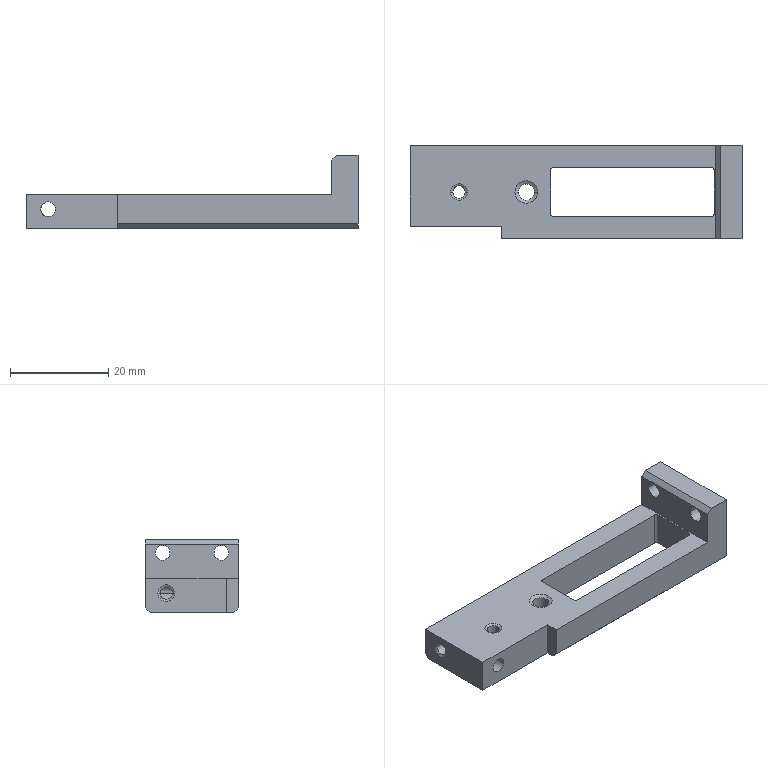Part | NX | 1 solid | 39 faces | box 67.7 x 19 x 15 mm | volume 6788 mm3 | plane 17 | cylinder 16 | cone 6 | commonest cylinder face diameters 3 x6 1 x4 2.5 x4 3.3 x2
STEP:
#1=CARTESIAN_POINT('',(-33.85,-7.,-3.5));
#2=VERTEX_POINT('',#1);
#3=CARTESIAN_POINT('',(-33.85,-7.,3.5));
#4=VERTEX_POINT('',#3);
#5=CARTESIAN_POINT('',(-33.85,-7.,0.));
#6=DIRECTION('',(0.,0.,1.));
#7=VECTOR('',#6,1000.);
#8=LINE('',#5,#7);
#9=EDGE_CURVE('',#2,#4,#8,.T.);
#10=ORIENTED_EDGE('',*,*,#9,.T.);
#11=CARTESIAN_POINT('',(-33.85,9.5,3.5));
#12=VERTEX_POINT('',#11);
#13=CARTESIAN_POINT('',(-33.85,0.,3.5));
#14=DIRECTION('',(0.,1.,0.));
#15=VECTOR('',#14,1000.);
#16=LINE('',#13,#15);
#17=EDGE_CURVE('',#4,#12,#16,.T.);
#18=ORIENTED_EDGE('',*,*,#17,.T.);
#19=CARTESIAN_POINT('',(-33.85,9.5,-2.5));
#20=VERTEX_POINT('',#19);
#21=CARTESIAN_POINT('',(-33.85,9.5,0.));
#22=DIRECTION('',(0.,0.,1.));
#23=VECTOR('',#22,1000.);
#24=LINE('',#21,#23);
#25=EDGE_CURVE('',#20,#12,#24,.T.);
#26=ORIENTED_EDGE('',*,*,#25,.F.);
#27=CARTESIAN_POINT('',(-33.85,8.5,-3.5));
#28=VERTEX_POINT('',#27);
#29=CARTESIAN_POINT('',(-33.85,12.,0.));
#30=DIRECTION('',(0.,0.7071,0.7071));
#31=VECTOR('',#30,1000.);
#32=LINE('',#29,#31);
#33=EDGE_CURVE('',#28,#20,#32,.T.);
#34=ORIENTED_EDGE('',*,*,#33,.F.);
#35=CARTESIAN_POINT('',(-33.85,0.,-3.5));
#36=DIRECTION('',(0.,1.,0.));
#37=VECTOR('',#36,1000.);
#38=LINE('',#35,#37);
#39=EDGE_CURVE('',#2,#28,#38,.T.);
#40=ORIENTED_EDGE('',*,*,#39,.F.);
#41=EDGE_LOOP('',(#10,#18,#26,#34,#40));
#42=FACE_BOUND('',#41,.T.);
#43=CARTESIAN_POINT('',(-33.85,6.95,0.5));
#44=VERTEX_POINT('',#43);
#45=CARTESIAN_POINT('',(-33.85,3.55,0.5));
#46=VERTEX_POINT('',#45);
#47=CARTESIAN_POINT('',(-33.85,5.25,0.5));
#48=DIRECTION('',(-1.,0.,0.));
#49=DIRECTION('',(0.,1.,0.));
#50=AXIS2_PLACEMENT_3D('',#47,#48,#49);
#51=CIRCLE('',#50,1.7);
#52=EDGE_CURVE('',#44,#46,#51,.T.);
#53=ORIENTED_EDGE('',*,*,#52,.F.);
#54=CARTESIAN_POINT('',(-33.85,5.25,0.5));
#55=DIRECTION('',(-1.,0.,0.));
#56=DIRECTION('',(0.,1.,0.));
#57=AXIS2_PLACEMENT_3D('',#54,#55,#56);
#58=CIRCLE('',#57,1.7);
#59=EDGE_CURVE('',#46,#44,#58,.T.);
#60=ORIENTED_EDGE('',*,*,#59,.F.);
#61=EDGE_LOOP('',(#53,#60));
#62=FACE_BOUND('',#61,.T.);
#63=CARTESIAN_POINT('',(-33.85,9.5,-3.5));
#64=DIRECTION('',(-1.,0.,0.));
#65=DIRECTION('',(0.,0.,1.));
#66=AXIS2_PLACEMENT_3D('',#63,#64,#65);
#67=PLANE('',#66);
#68=ADVANCED_FACE('',(#42,#62),#67,.T.);
#69=CARTESIAN_POINT('',(-15.15,-7.,-3.5));
#70=VERTEX_POINT('',#69);
#71=CARTESIAN_POINT('',(-15.15,-8.5,-3.5));
#72=VERTEX_POINT('',#71);
#73=CARTESIAN_POINT('',(-15.15,0.,-3.5));
#74=DIRECTION('',(0.,-1.,0.));
#75=VECTOR('',#74,1000.);
#76=LINE('',#73,#75);
#77=EDGE_CURVE('',#70,#72,#76,.T.);
#78=ORIENTED_EDGE('',*,*,#77,.T.);
#79=CARTESIAN_POINT('',(-15.15,-9.5,-2.5));
#80=VERTEX_POINT('',#79);
#81=CARTESIAN_POINT('',(-15.15,-9.5,-2.5));
#82=DIRECTION('',(0.,0.7071,-0.7071));
#83=VECTOR('',#82,1000.);
#84=LINE('',#81,#83);
#85=EDGE_CURVE('',#80,#72,#84,.T.);
#86=ORIENTED_EDGE('',*,*,#85,.F.);
#87=CARTESIAN_POINT('',(-15.15,-9.5,3.5));
#88=VERTEX_POINT('',#87);
#89=CARTESIAN_POINT('',(-15.15,-9.5,3.5));
#90=DIRECTION('',(0.,0.,-1.));
#91=VECTOR('',#90,1000.);
#92=LINE('',#89,#91);
#93=EDGE_CURVE('',#88,#80,#92,.T.);
#94=ORIENTED_EDGE('',*,*,#93,.F.);
#95=CARTESIAN_POINT('',(-15.15,-7.,3.5));
#96=VERTEX_POINT('',#95);
#97=CARTESIAN_POINT('',(-15.15,0.,3.5));
#98=DIRECTION('',(0.,-1.,0.));
#99=VECTOR('',#98,1000.);
#100=LINE('',#97,#99);
#101=EDGE_CURVE('',#96,#88,#100,.T.);
#102=ORIENTED_EDGE('',*,*,#101,.F.);
#103=CARTESIAN_POINT('',(-15.15,-7.,-3.5));
#104=DIRECTION('',(0.,0.,1.));
#105=VECTOR('',#104,1000.);
#106=LINE('',#103,#105);
#107=EDGE_CURVE('',#70,#96,#106,.T.);
#108=ORIENTED_EDGE('',*,*,#107,.F.);
#109=EDGE_LOOP('',(#78,#86,#94,#102,#108));
#110=FACE_BOUND('',#109,.T.);
#111=CARTESIAN_POINT('',(-15.15,-9.5,3.5));
#112=DIRECTION('',(1.,0.,0.));
#113=DIRECTION('',(0.,1.,0.));
#114=AXIS2_PLACEMENT_3D('',#111,#112,#113);
#115=PLANE('',#114);
#116=ADVANCED_FACE('',(#110),#115,.F.);
#117=CARTESIAN_POINT('',(33.85,8.5,-3.5));
#118=VERTEX_POINT('',#117);
#119=CARTESIAN_POINT('',(0.,8.5,-3.5));
#120=DIRECTION('',(1.,0.,0.));
#121=VECTOR('',#120,1000.);
#122=LINE('',#119,#121);
#123=EDGE_CURVE('',#28,#118,#122,.T.);
#124=ORIENTED_EDGE('',*,*,#123,.T.);
#125=CARTESIAN_POINT('',(33.85,-8.5,-3.5));
#126=VERTEX_POINT('',#125);
#127=CARTESIAN_POINT('',(33.85,0.,-3.5));
#128=DIRECTION('',(0.,1.,0.));
#129=VECTOR('',#128,1000.);
#130=LINE('',#127,#129);
#131=EDGE_CURVE('',#126,#118,#130,.T.);
#132=ORIENTED_EDGE('',*,*,#131,.F.);
#133=CARTESIAN_POINT('',(0.,-8.5,-3.5));
#134=DIRECTION('',(-1.,0.,0.));
#135=VECTOR('',#134,1000.);
#136=LINE('',#133,#135);
#137=EDGE_CURVE('',#126,#72,#136,.T.);
#138=ORIENTED_EDGE('',*,*,#137,.T.);
#139=ORIENTED_EDGE('',*,*,#77,.F.);
#140=CARTESIAN_POINT('',(0.,-7.,-3.5));
#141=DIRECTION('',(1.,0.,0.));
#142=VECTOR('',#141,1000.);
#143=LINE('',#140,#142);
#144=EDGE_CURVE('',#2,#70,#143,.T.);
#145=ORIENTED_EDGE('',*,*,#144,.F.);
#146=ORIENTED_EDGE('',*,*,#39,.T.);
#147=EDGE_LOOP('',(#124,#132,#138,#139,#145,#146));
#148=FACE_BOUND('',#147,.T.);
#149=CARTESIAN_POINT('',(27.65,-5.,-3.5));
#150=VERTEX_POINT('',#149);
#151=CARTESIAN_POINT('',(-4.65,-5.,-3.5));
#152=VERTEX_POINT('',#151);
#153=CARTESIAN_POINT('',(0.,-5.,-3.5));
#154=DIRECTION('',(-1.,0.,0.));
#155=VECTOR('',#154,1000.);
#156=LINE('',#153,#155);
#157=EDGE_CURVE('',#150,#152,#156,.T.);
#158=ORIENTED_EDGE('',*,*,#157,.F.);
#159=CARTESIAN_POINT('',(28.15,-4.5,-3.5));
#160=VERTEX_POINT('',#159);
#161=CARTESIAN_POINT('',(27.65,-4.5,-3.5));
#162=DIRECTION('',(0.,0.,1.));
#163=DIRECTION('',(0.,1.,0.));
#164=AXIS2_PLACEMENT_3D('',#161,#162,#163);
#165=CIRCLE('',#164,0.5);
#166=EDGE_CURVE('',#150,#160,#165,.T.);
#167=ORIENTED_EDGE('',*,*,#166,.T.);
#168=CARTESIAN_POINT('',(28.15,4.5,-3.5));
#169=VERTEX_POINT('',#168);
#170=CARTESIAN_POINT('',(28.15,0.,-3.5));
#171=DIRECTION('',(0.,-1.,0.));
#172=VECTOR('',#171,1000.);
#173=LINE('',#170,#172);
#174=EDGE_CURVE('',#169,#160,#173,.T.);
#175=ORIENTED_EDGE('',*,*,#174,.F.);
#176=CARTESIAN_POINT('',(27.65,5.,-3.5));
#177=VERTEX_POINT('',#176);
#178=CARTESIAN_POINT('',(27.65,4.5,-3.5));
#179=DIRECTION('',(0.,0.,1.));
#180=DIRECTION('',(0.,1.,0.));
#181=AXIS2_PLACEMENT_3D('',#178,#179,#180);
#182=CIRCLE('',#181,0.5);
#183=EDGE_CURVE('',#169,#177,#182,.T.);
#184=ORIENTED_EDGE('',*,*,#183,.T.);
#185=CARTESIAN_POINT('',(-4.65,5.,-3.5));
#186=VERTEX_POINT('',#185);
#187=CARTESIAN_POINT('',(0.,5.,-3.5));
#188=DIRECTION('',(1.,0.,0.));
#189=VECTOR('',#188,1000.);
#190=LINE('',#187,#189);
#191=EDGE_CURVE('',#186,#177,#190,.T.);
#192=ORIENTED_EDGE('',*,*,#191,.F.);
#193=CARTESIAN_POINT('',(-5.15,4.5,-3.5));
#194=VERTEX_POINT('',#193);
#195=CARTESIAN_POINT('',(-4.65,4.5,-3.5));
#196=DIRECTION('',(0.,0.,1.));
#197=DIRECTION('',(0.,1.,0.));
#198=AXIS2_PLACEMENT_3D('',#195,#196,#197);
#199=CIRCLE('',#198,0.5);
#200=EDGE_CURVE('',#186,#194,#199,.T.);
#201=ORIENTED_EDGE('',*,*,#200,.T.);
#202=CARTESIAN_POINT('',(-5.15,-4.5,-3.5));
#203=VERTEX_POINT('',#202);
#204=CARTESIAN_POINT('',(-5.15,0.,-3.5));
#205=DIRECTION('',(0.,1.,0.));
#206=VECTOR('',#205,1000.);
#207=LINE('',#204,#206);
#208=EDGE_CURVE('',#203,#194,#207,.T.);
#209=ORIENTED_EDGE('',*,*,#208,.F.);
#210=CARTESIAN_POINT('',(-4.65,-4.5,-3.5));
#211=DIRECTION('',(0.,0.,1.));
#212=DIRECTION('',(0.,1.,0.));
#213=AXIS2_PLACEMENT_3D('',#210,#211,#212);
#214=CIRCLE('',#213,0.5);
#215=EDGE_CURVE('',#203,#152,#214,.T.);
#216=ORIENTED_EDGE('',*,*,#215,.T.);
#217=EDGE_LOOP('',(#158,#167,#175,#184,#192,#201,#209,#216));
#218=FACE_BOUND('',#217,.T.);
#219=CARTESIAN_POINT('',(-22.6,0.,-3.5));
#220=VERTEX_POINT('',#219);
#221=CARTESIAN_POINT('',(-25.1,0.,-3.5));
#222=VERTEX_POINT('',#221);
#223=CARTESIAN_POINT('',(-23.85,0.,-3.5));
#224=DIRECTION('',(0.,0.,1.));
#225=DIRECTION('',(1.,0.,0.));
#226=AXIS2_PLACEMENT_3D('',#223,#224,#225);
#227=CIRCLE('',#226,1.25);
#228=EDGE_CURVE('',#220,#222,#227,.T.);
#229=ORIENTED_EDGE('',*,*,#228,.T.);
#230=CARTESIAN_POINT('',(-23.85,0.,-3.5));
#231=DIRECTION('',(0.,0.,1.));
#232=DIRECTION('',(1.,0.,0.));
#233=AXIS2_PLACEMENT_3D('',#230,#231,#232);
#234=CIRCLE('',#233,1.25);
#235=EDGE_CURVE('',#222,#220,#234,.T.);
#236=ORIENTED_EDGE('',*,*,#235,.T.);
#237=EDGE_LOOP('',(#229,#236));
#238=FACE_BOUND('',#237,.T.);
#239=CARTESIAN_POINT('',(-11.8,0.,-3.5));
#240=VERTEX_POINT('',#239);
#241=CARTESIAN_POINT('',(-8.5,0.,-3.5));
#242=VERTEX_POINT('',#241);
#243=CARTESIAN_POINT('',(-10.15,0.,-3.5));
#244=DIRECTION('',(0.,0.,1.));
#245=DIRECTION('',(1.,0.,0.));
#246=AXIS2_PLACEMENT_3D('',#243,#244,#245);
#247=CIRCLE('',#246,1.65);
#248=EDGE_CURVE('',#240,#242,#247,.T.);
#249=ORIENTED_EDGE('',*,*,#248,.T.);
#250=CARTESIAN_POINT('',(-10.15,0.,-3.5));
#251=DIRECTION('',(0.,0.,1.));
#252=DIRECTION('',(1.,0.,0.));
#253=AXIS2_PLACEMENT_3D('',#250,#251,#252);
#254=CIRCLE('',#253,1.65);
#255=EDGE_CURVE('',#242,#240,#254,.T.);
#256=ORIENTED_EDGE('',*,*,#255,.T.);
#257=EDGE_LOOP('',(#249,#256));
#258=FACE_BOUND('',#257,.T.);
#259=CARTESIAN_POINT('',(0.,0.,-3.5));
#260=DIRECTION('',(0.,0.,1.));
#261=DIRECTION('',(1.,0.,0.));
#262=AXIS2_PLACEMENT_3D('',#259,#260,#261);
#263=PLANE('',#262);
#264=ADVANCED_FACE('',(#148,#218,#238,#258),#263,.F.);
#265=CARTESIAN_POINT('',(28.5,9.5,3.5));
#266=VERTEX_POINT('',#265);
#267=CARTESIAN_POINT('',(28.5,-9.5,3.5));
#268=VERTEX_POINT('',#267);
#269=CARTESIAN_POINT('',(28.5,0.,3.5));
#270=DIRECTION('',(0.,-1.,0.));
#271=VECTOR('',#270,1000.);
#272=LINE('',#269,#271);
#273=EDGE_CURVE('',#266,#268,#272,.T.);
#274=ORIENTED_EDGE('',*,*,#273,.T.);
#275=CARTESIAN_POINT('',(28.5,-9.5,10.5));
#276=VERTEX_POINT('',#275);
#277=CARTESIAN_POINT('',(28.5,-9.5,0.));
#278=DIRECTION('',(0.,0.,-1.));
#279=VECTOR('',#278,1000.);
#280=LINE('',#277,#279);
#281=EDGE_CURVE('',#276,#268,#280,.T.);
#282=ORIENTED_EDGE('',*,*,#281,.F.);
#283=CARTESIAN_POINT('',(28.5,9.5,10.5));
#284=VERTEX_POINT('',#283);
#285=CARTESIAN_POINT('',(28.5,0.,10.5));
#286=DIRECTION('',(0.,1.,0.));
#287=VECTOR('',#286,1000.);
#288=LINE('',#285,#287);
#289=EDGE_CURVE('',#276,#284,#288,.T.);
#290=ORIENTED_EDGE('',*,*,#289,.T.);
#291=CARTESIAN_POINT('',(28.5,9.5,0.));
#292=DIRECTION('',(0.,0.,1.));
#293=VECTOR('',#292,1000.);
#294=LINE('',#291,#293);
#295=EDGE_CURVE('',#266,#284,#294,.T.);
#296=ORIENTED_EDGE('',*,*,#295,.F.);
#297=EDGE_LOOP('',(#274,#282,#290,#296));
#298=FACE_BOUND('',#297,.T.);
#299=CARTESIAN_POINT('',(28.5,-4.5,8.73));
#300=VERTEX_POINT('',#299);
#301=CARTESIAN_POINT('',(28.5,-7.5,8.73));
#302=VERTEX_POINT('',#301);
#303=CARTESIAN_POINT('',(28.5,-6.,8.73));
#304=DIRECTION('',(1.,0.,0.));
#305=DIRECTION('',(0.,1.,0.));
#306=AXIS2_PLACEMENT_3D('',#303,#304,#305);
#307=CIRCLE('',#306,1.5);
#308=EDGE_CURVE('',#300,#302,#307,.T.);
#309=ORIENTED_EDGE('',*,*,#308,.T.);
#310=CARTESIAN_POINT('',(28.5,-6.,8.73));
#311=DIRECTION('',(1.,0.,0.));
#312=DIRECTION('',(0.,1.,0.));
#313=AXIS2_PLACEMENT_3D('',#310,#311,#312);
#314=CIRCLE('',#313,1.5);
#315=EDGE_CURVE('',#302,#300,#314,.T.);
#316=ORIENTED_EDGE('',*,*,#315,.T.);
#317=EDGE_LOOP('',(#309,#316));
#318=FACE_BOUND('',#317,.T.);
#319=CARTESIAN_POINT('',(28.5,7.5,8.73));
#320=VERTEX_POINT('',#319);
#321=CARTESIAN_POINT('',(28.5,4.5,8.73));
#322=VERTEX_POINT('',#321);
#323=CARTESIAN_POINT('',(28.5,6.,8.73));
#324=DIRECTION('',(1.,0.,0.));
#325=DIRECTION('',(0.,1.,0.));
#326=AXIS2_PLACEMENT_3D('',#323,#324,#325);
#327=CIRCLE('',#326,1.5);
#328=EDGE_CURVE('',#320,#322,#327,.T.);
#329=ORIENTED_EDGE('',*,*,#328,.T.);
#330=CARTESIAN_POINT('',(28.5,6.,8.73));
#331=DIRECTION('',(1.,0.,0.));
#332=DIRECTION('',(0.,1.,0.));
#333=AXIS2_PLACEMENT_3D('',#330,#331,#332);
#334=CIRCLE('',#333,1.5);
#335=EDGE_CURVE('',#322,#320,#334,.T.);
#336=ORIENTED_EDGE('',*,*,#335,.T.);
#337=EDGE_LOOP('',(#329,#336));
#338=FACE_BOUND('',#337,.T.);
#339=CARTESIAN_POINT('',(28.5,9.5,3.5));
#340=DIRECTION('',(-1.,0.,0.));
#341=DIRECTION('',(0.,0.,1.));
#342=AXIS2_PLACEMENT_3D('',#339,#340,#341);
#343=PLANE('',#342);
#344=ADVANCED_FACE('',(#298,#318,#338),#343,.T.);
#345=ORIENTED_EDGE('',*,*,#101,.T.);
#346=CARTESIAN_POINT('',(0.,-9.5,3.5));
#347=DIRECTION('',(-1.,0.,0.));
#348=VECTOR('',#347,1000.);
#349=LINE('',#346,#348);
#350=EDGE_CURVE('',#268,#88,#349,.T.);
#351=ORIENTED_EDGE('',*,*,#350,.F.);
#352=ORIENTED_EDGE('',*,*,#273,.F.);
#353=CARTESIAN_POINT('',(0.,9.5,3.5));
#354=DIRECTION('',(1.,0.,0.));
#355=VECTOR('',#354,1000.);
#356=LINE('',#353,#355);
#357=EDGE_CURVE('',#12,#266,#356,.T.);
#358=ORIENTED_EDGE('',*,*,#357,.F.);
#359=ORIENTED_EDGE('',*,*,#17,.F.);
#360=CARTESIAN_POINT('',(0.,-7.,3.5));
#361=DIRECTION('',(1.,0.,0.));
#362=VECTOR('',#361,1000.);
#363=LINE('',#360,#362);
#364=EDGE_CURVE('',#4,#96,#363,.T.);
#365=ORIENTED_EDGE('',*,*,#364,.T.);
#366=EDGE_LOOP('',(#345,#351,#352,#358,#359,#365));
#367=FACE_BOUND('',#366,.T.);
#368=CARTESIAN_POINT('',(27.65,-5.,3.5));
#369=VERTEX_POINT('',#368);
#370=CARTESIAN_POINT('',(-4.65,-5.,3.5));
#371=VERTEX_POINT('',#370);
#372=CARTESIAN_POINT('',(0.,-5.,3.5));
#373=DIRECTION('',(-1.,0.,0.));
#374=VECTOR('',#373,1000.);
#375=LINE('',#372,#374);
#376=EDGE_CURVE('',#369,#371,#375,.T.);
#377=ORIENTED_EDGE('',*,*,#376,.T.);
#378=CARTESIAN_POINT('',(-5.15,-4.5,3.5));
#379=VERTEX_POINT('',#378);
#380=CARTESIAN_POINT('',(-4.65,-4.5,3.5));
#381=DIRECTION('',(0.,0.,1.));
#382=DIRECTION('',(0.,1.,0.));
#383=AXIS2_PLACEMENT_3D('',#380,#381,#382);
#384=CIRCLE('',#383,0.5);
#385=EDGE_CURVE('',#379,#371,#384,.T.);
#386=ORIENTED_EDGE('',*,*,#385,.F.);
#387=CARTESIAN_POINT('',(-5.15,4.5,3.5));
#388=VERTEX_POINT('',#387);
#389=CARTESIAN_POINT('',(-5.15,0.,3.5));
#390=DIRECTION('',(0.,1.,0.));
#391=VECTOR('',#390,1000.);
#392=LINE('',#389,#391);
#393=EDGE_CURVE('',#379,#388,#392,.T.);
#394=ORIENTED_EDGE('',*,*,#393,.T.);
#395=CARTESIAN_POINT('',(-4.65,5.,3.5));
#396=VERTEX_POINT('',#395);
#397=CARTESIAN_POINT('',(-4.65,4.5,3.5));
#398=DIRECTION('',(0.,0.,1.));
#399=DIRECTION('',(0.,1.,0.));
#400=AXIS2_PLACEMENT_3D('',#397,#398,#399);
#401=CIRCLE('',#400,0.5);
#402=EDGE_CURVE('',#396,#388,#401,.T.);
#403=ORIENTED_EDGE('',*,*,#402,.F.);
#404=CARTESIAN_POINT('',(27.65,5.,3.5));
#405=VERTEX_POINT('',#404);
#406=CARTESIAN_POINT('',(0.,5.,3.5));
#407=DIRECTION('',(1.,0.,0.));
#408=VECTOR('',#407,1000.);
#409=LINE('',#406,#408);
#410=EDGE_CURVE('',#396,#405,#409,.T.);
#411=ORIENTED_EDGE('',*,*,#410,.T.);
#412=CARTESIAN_POINT('',(28.15,4.5,3.5));
#413=VERTEX_POINT('',#412);
#414=CARTESIAN_POINT('',(27.65,4.5,3.5));
#415=DIRECTION('',(0.,0.,1.));
#416=DIRECTION('',(0.,1.,0.));
#417=AXIS2_PLACEMENT_3D('',#414,#415,#416);
#418=CIRCLE('',#417,0.5);
#419=EDGE_CURVE('',#413,#405,#418,.T.);
#420=ORIENTED_EDGE('',*,*,#419,.F.);
#421=CARTESIAN_POINT('',(28.15,-4.5,3.5));
#422=VERTEX_POINT('',#421);
#423=CARTESIAN_POINT('',(28.15,0.,3.5));
#424=DIRECTION('',(0.,-1.,0.));
#425=VECTOR('',#424,1000.);
#426=LINE('',#423,#425);
#427=EDGE_CURVE('',#413,#422,#426,.T.);
#428=ORIENTED_EDGE('',*,*,#427,.T.);
#429=CARTESIAN_POINT('',(27.65,-4.5,3.5));
#430=DIRECTION('',(0.,0.,1.));
#431=DIRECTION('',(0.,1.,0.));
#432=AXIS2_PLACEMENT_3D('',#429,#430,#431);
#433=CIRCLE('',#432,0.5);
#434=EDGE_CURVE('',#369,#422,#433,.T.);
#435=ORIENTED_EDGE('',*,*,#434,.F.);
#436=EDGE_LOOP('',(#377,#386,#394,#403,#411,#420,#428,#435));
#437=FACE_BOUND('',#436,.T.);
#438=CARTESIAN_POINT('',(-12.465,0.,3.5));
#439=VERTEX_POINT('',#438);
#440=CARTESIAN_POINT('',(-7.835,0.,3.5));
#441=VERTEX_POINT('',#440);
#442=CARTESIAN_POINT('',(-10.15,0.,3.5));
#443=DIRECTION('',(0.,0.,1.));
#444=DIRECTION('',(1.,0.,0.));
#445=AXIS2_PLACEMENT_3D('',#442,#443,#444);
#446=CIRCLE('',#445,2.315);
#447=EDGE_CURVE('',#439,#441,#446,.T.);
#448=ORIENTED_EDGE('',*,*,#447,.F.);
#449=CARTESIAN_POINT('',(-10.15,0.,3.5));
#450=DIRECTION('',(0.,0.,1.));
#451=DIRECTION('',(1.,0.,0.));
#452=AXIS2_PLACEMENT_3D('',#449,#450,#451);
#453=CIRCLE('',#452,2.315);
#454=EDGE_CURVE('',#441,#439,#453,.T.);
#455=ORIENTED_EDGE('',*,*,#454,.F.);
#456=EDGE_LOOP('',(#448,#455));
#457=FACE_BOUND('',#456,.T.);
#458=CARTESIAN_POINT('',(-22.15,0.,3.5));
#459=VERTEX_POINT('',#458);
#460=CARTESIAN_POINT('',(-25.55,0.,3.5));
#461=VERTEX_POINT('',#460);
#462=CARTESIAN_POINT('',(-23.85,0.,3.5));
#463=DIRECTION('',(0.,0.,1.));
#464=DIRECTION('',(1.,0.,0.));
#465=AXIS2_PLACEMENT_3D('',#462,#463,#464);
#466=CIRCLE('',#465,1.7);
#467=EDGE_CURVE('',#459,#461,#466,.T.);
#468=ORIENTED_EDGE('',*,*,#467,.F.);
#469=CARTESIAN_POINT('',(-23.85,0.,3.5));
#470=DIRECTION('',(0.,0.,1.));
#471=DIRECTION('',(1.,0.,0.));
#472=AXIS2_PLACEMENT_3D('',#469,#470,#471);
#473=CIRCLE('',#472,1.7);
#474=EDGE_CURVE('',#461,#459,#473,.T.);
#475=ORIENTED_EDGE('',*,*,#474,.F.);
#476=EDGE_LOOP('',(#468,#475));
#477=FACE_BOUND('',#476,.T.);
#478=CARTESIAN_POINT('',(0.,0.,3.5));
#479=DIRECTION('',(0.,0.,1.));
#480=DIRECTION('',(1.,0.,0.));
#481=AXIS2_PLACEMENT_3D('',#478,#479,#480);
#482=PLANE('',#481);
#483=ADVANCED_FACE('',(#367,#437,#457,#477),#482,.T.);
#484=CARTESIAN_POINT('',(-30.85,6.5,0.5));
#485=VERTEX_POINT('',#484);
#486=CARTESIAN_POINT('',(-30.85,4.,0.5));
#487=VERTEX_POINT('',#486);
#488=CARTESIAN_POINT('',(-30.85,6.5,0.5));
#489=CARTESIAN_POINT('',(-30.85,6.5,0.6667));
#490=CARTESIAN_POINT('',(-30.788,6.424,0.9601));
#491=CARTESIAN_POINT('',(-30.695,6.313,1.179));
#492=CARTESIAN_POINT('',(-30.552,6.12,1.4));
#493=CARTESIAN_POINT('',(-30.532,6.094,1.425));
#494=CARTESIAN_POINT('',(-30.389,5.883,1.59));
#495=CARTESIAN_POINT('',(-30.285,5.699,1.674));
#496=CARTESIAN_POINT('',(-30.109,5.25,1.801));
#497=CARTESIAN_POINT('',(-30.284,4.802,1.674));
#498=CARTESIAN_POINT('',(-30.39,4.616,1.589));
#499=CARTESIAN_POINT('',(-30.53,4.408,1.427));
#500=CARTESIAN_POINT('',(-30.553,4.379,1.399));
#501=CARTESIAN_POINT('',(-30.695,4.187,1.18));
#502=CARTESIAN_POINT('',(-30.788,4.076,0.9605));
#503=CARTESIAN_POINT('',(-30.85,4.,0.6669));
#504=CARTESIAN_POINT('',(-30.85,4.,0.5));
#505=B_SPLINE_CURVE_WITH_KNOTS('',3,(#488,#489,#490,#491,#492,#493,#494,#495,#496,#497,#498,#499,#500,#501,#502,#503,#504),.UNSPECIFIED.,.F.,.F.,(4,1,1,1,1,1,1,1,1,1,1,1,1,1,4),(0.,0.125,0.1875,0.25,0.2812,0.3125,0.375,0.5,0.625,0.6875,0.7188,0.75,0.8125,0.875,1.),.UNSPECIFIED.);
#506=EDGE_CURVE('',#485,#487,#505,.T.);
#507=ORIENTED_EDGE('',*,*,#506,.T.);
#508=CARTESIAN_POINT('',(-33.59,4.,0.5));
#509=VERTEX_POINT('',#508);
#510=CARTESIAN_POINT('',(-33.85,4.,0.5));
#511=DIRECTION('',(-1.,0.,0.));
#512=VECTOR('',#511,1000.);
#513=LINE('',#510,#512);
#514=EDGE_CURVE('',#487,#509,#513,.T.);
#515=ORIENTED_EDGE('',*,*,#514,.T.);
#516=CARTESIAN_POINT('',(-33.59,6.5,0.5));
#517=VERTEX_POINT('',#516);
#518=CARTESIAN_POINT('',(-33.59,5.25,0.5));
#519=DIRECTION('',(-1.,0.,0.));
#520=DIRECTION('',(0.,1.,0.));
#521=AXIS2_PLACEMENT_3D('',#518,#519,#520);
#522=CIRCLE('',#521,1.25);
#523=EDGE_CURVE('',#509,#517,#522,.T.);
#524=ORIENTED_EDGE('',*,*,#523,.T.);
#525=CARTESIAN_POINT('',(-33.85,6.5,0.5));
#526=DIRECTION('',(-1.,0.,0.));
#527=VECTOR('',#526,1000.);
#528=LINE('',#525,#527);
#529=EDGE_CURVE('',#485,#517,#528,.T.);
#530=ORIENTED_EDGE('',*,*,#529,.F.);
#531=EDGE_LOOP('',(#507,#515,#524,#530));
#532=FACE_BOUND('',#531,.T.);
#533=CARTESIAN_POINT('',(-33.85,5.25,0.5));
#534=DIRECTION('',(-1.,0.,0.));
#535=DIRECTION('',(0.,1.,0.));
#536=AXIS2_PLACEMENT_3D('',#533,#534,#535);
#537=CYLINDRICAL_SURFACE('',#536,1.25);
#538=ADVANCED_FACE('',(#532),#537,.F.);
#539=ORIENTED_EDGE('',*,*,#52,.T.);
#540=CARTESIAN_POINT('',(-33.59,4.,0.5));
#541=DIRECTION('',(-0.5,-0.866,0.));
#542=VECTOR('',#541,1000.);
#543=LINE('',#540,#542);
#544=EDGE_CURVE('',#46,#509,#543,.F.);
#545=ORIENTED_EDGE('',*,*,#544,.T.);
#546=CARTESIAN_POINT('',(-33.59,5.25,0.5));
#547=DIRECTION('',(-1.,0.,0.));
#548=DIRECTION('',(0.,1.,0.));
#549=AXIS2_PLACEMENT_3D('',#546,#547,#548);
#550=CIRCLE('',#549,1.25);
#551=EDGE_CURVE('',#517,#509,#550,.T.);
#552=ORIENTED_EDGE('',*,*,#551,.F.);
#553=CARTESIAN_POINT('',(-33.59,6.5,0.5));
#554=DIRECTION('',(-0.5,0.866,0.));
#555=VECTOR('',#554,1000.);
#556=LINE('',#553,#555);
#557=EDGE_CURVE('',#44,#517,#556,.F.);
#558=ORIENTED_EDGE('',*,*,#557,.F.);
#559=EDGE_LOOP('',(#539,#545,#552,#558));
#560=FACE_BOUND('',#559,.T.);
#561=CARTESIAN_POINT('',(-33.59,5.25,0.5));
#562=DIRECTION('',(-1.,0.,0.));
#563=DIRECTION('',(0.,1.,0.));
#564=AXIS2_PLACEMENT_3D('',#561,#562,#563);
#565=CONICAL_SURFACE('',#564,1.25,1.047);
#566=ADVANCED_FACE('',(#560),#565,.F.);
#567=CARTESIAN_POINT('',(33.85,9.5,-2.5));
#568=VERTEX_POINT('',#567);
#569=CARTESIAN_POINT('',(0.,9.5,-2.5));
#570=DIRECTION('',(1.,0.,0.));
#571=VECTOR('',#570,1000.);
#572=LINE('',#569,#571);
#573=EDGE_CURVE('',#20,#568,#572,.T.);
#574=ORIENTED_EDGE('',*,*,#573,.F.);
#575=ORIENTED_EDGE('',*,*,#25,.T.);
#576=ORIENTED_EDGE('',*,*,#357,.T.);
#577=ORIENTED_EDGE('',*,*,#295,.T.);
#578=CARTESIAN_POINT('',(29.5,9.5,11.5));
#579=VERTEX_POINT('',#578);
#580=CARTESIAN_POINT('',(18.,9.5,0.));
#581=DIRECTION('',(0.7071,0.,0.7071));
#582=VECTOR('',#581,1000.);
#583=LINE('',#580,#582);
#584=EDGE_CURVE('',#284,#579,#583,.T.);
#585=ORIENTED_EDGE('',*,*,#584,.T.);
#586=CARTESIAN_POINT('',(33.85,9.5,11.5));
#587=VERTEX_POINT('',#586);
#588=CARTESIAN_POINT('',(0.,9.5,11.5));
#589=DIRECTION('',(-1.,0.,0.));
#590=VECTOR('',#589,1000.);
#591=LINE('',#588,#590);
#592=EDGE_CURVE('',#587,#579,#591,.T.);
#593=ORIENTED_EDGE('',*,*,#592,.F.);
#594=CARTESIAN_POINT('',(33.85,9.5,0.));
#595=DIRECTION('',(0.,0.,-1.));
#596=VECTOR('',#595,1000.);
#597=LINE('',#594,#596);
#598=EDGE_CURVE('',#587,#568,#597,.T.);
#599=ORIENTED_EDGE('',*,*,#598,.T.);
#600=EDGE_LOOP('',(#574,#575,#576,#577,#585,#593,#599));
#601=FACE_BOUND('',#600,.T.);
#602=CARTESIAN_POINT('',(-30.85,9.5,0.5));
#603=VERTEX_POINT('',#602);
#604=CARTESIAN_POINT('',(-27.85,9.5,0.5));
#605=VERTEX_POINT('',#604);
#606=CARTESIAN_POINT('',(-29.35,9.5,0.5));
#607=DIRECTION('',(0.,1.,0.));
#608=DIRECTION('',(-1.,0.,0.));
#609=AXIS2_PLACEMENT_3D('',#606,#607,#608);
#610=CIRCLE('',#609,1.5);
#611=EDGE_CURVE('',#603,#605,#610,.T.);
#612=ORIENTED_EDGE('',*,*,#611,.F.);
#613=CARTESIAN_POINT('',(-29.35,9.5,0.5));
#614=DIRECTION('',(0.,1.,0.));
#615=DIRECTION('',(-1.,0.,0.));
#616=AXIS2_PLACEMENT_3D('',#613,#614,#615);
#617=CIRCLE('',#616,1.5);
#618=EDGE_CURVE('',#605,#603,#617,.T.);
#619=ORIENTED_EDGE('',*,*,#618,.F.);
#620=EDGE_LOOP('',(#612,#619));
#621=FACE_BOUND('',#620,.T.);
#622=CARTESIAN_POINT('',(33.85,9.5,-3.5));
#623=DIRECTION('',(0.,1.,0.));
#624=DIRECTION('',(1.,0.,0.));
#625=AXIS2_PLACEMENT_3D('',#622,#623,#624);
#626=PLANE('',#625);
#627=ADVANCED_FACE('',(#601,#621),#626,.T.);
#628=ORIENTED_EDGE('',*,*,#93,.T.);
#629=CARTESIAN_POINT('',(33.85,-9.5,-2.5));
#630=VERTEX_POINT('',#629);
#631=CARTESIAN_POINT('',(33.85,-9.5,-2.5));
#632=DIRECTION('',(-1.,0.,0.));
#633=VECTOR('',#632,1000.);
#634=LINE('',#631,#633);
#635=EDGE_CURVE('',#630,#80,#634,.T.);
#636=ORIENTED_EDGE('',*,*,#635,.F.);
#637=CARTESIAN_POINT('',(33.85,-9.5,11.5));
#638=VERTEX_POINT('',#637);
#639=CARTESIAN_POINT('',(33.85,-9.5,0.));
#640=DIRECTION('',(0.,0.,1.));
#641=VECTOR('',#640,1000.);
#642=LINE('',#639,#641);
#643=EDGE_CURVE('',#630,#638,#642,.T.);
#644=ORIENTED_EDGE('',*,*,#643,.T.);
#645=CARTESIAN_POINT('',(29.5,-9.5,11.5));
#646=VERTEX_POINT('',#645);
#647=CARTESIAN_POINT('',(33.85,-9.5,11.5));
#648=DIRECTION('',(-1.,0.,0.));
#649=VECTOR('',#648,1000.);
#650=LINE('',#647,#649);
#651=EDGE_CURVE('',#638,#646,#650,.T.);
#652=ORIENTED_EDGE('',*,*,#651,.T.);
#653=CARTESIAN_POINT('',(28.5,-9.5,10.5));
#654=DIRECTION('',(0.7071,0.,0.7071));
#655=VECTOR('',#654,1000.);
#656=LINE('',#653,#655);
#657=EDGE_CURVE('',#276,#646,#656,.T.);
#658=ORIENTED_EDGE('',*,*,#657,.F.);
#659=ORIENTED_EDGE('',*,*,#281,.T.);
#660=ORIENTED_EDGE('',*,*,#350,.T.);
#661=EDGE_LOOP('',(#628,#636,#644,#652,#658,#659,#660));
#662=FACE_BOUND('',#661,.T.);
#663=CARTESIAN_POINT('',(-33.85,-9.5,-3.5));
#664=DIRECTION('',(0.,-1.,0.));
#665=DIRECTION('',(0.,0.,-1.));
#666=AXIS2_PLACEMENT_3D('',#663,#664,#665);
#667=PLANE('',#666);
#668=ADVANCED_FACE('',(#662),#667,.T.);
#669=ORIENTED_EDGE('',*,*,#598,.F.);
#670=CARTESIAN_POINT('',(33.85,0.,11.5));
#671=DIRECTION('',(0.,1.,0.));
#672=VECTOR('',#671,1000.);
#673=LINE('',#670,#672);
#674=EDGE_CURVE('',#638,#587,#673,.T.);
#675=ORIENTED_EDGE('',*,*,#674,.F.);
#676=ORIENTED_EDGE('',*,*,#643,.F.);
#677=CARTESIAN_POINT('',(33.85,-12.,0.));
#678=DIRECTION('',(0.,-0.7071,0.7071));
#679=VECTOR('',#678,1000.);
#680=LINE('',#677,#679);
#681=EDGE_CURVE('',#126,#630,#680,.T.);
#682=ORIENTED_EDGE('',*,*,#681,.F.);
#683=ORIENTED_EDGE('',*,*,#131,.T.);
#684=CARTESIAN_POINT('',(33.85,12.,0.));
#685=DIRECTION('',(0.,-0.7071,-0.7071));
#686=VECTOR('',#685,1000.);
#687=LINE('',#684,#686);
#688=EDGE_CURVE('',#568,#118,#687,.T.);
#689=ORIENTED_EDGE('',*,*,#688,.F.);
#690=EDGE_LOOP('',(#669,#675,#676,#682,#683,#689));
#691=FACE_BOUND('',#690,.T.);
#692=CARTESIAN_POINT('',(33.85,-4.5,8.73));
#693=VERTEX_POINT('',#692);
#694=CARTESIAN_POINT('',(33.85,-7.5,8.73));
#695=VERTEX_POINT('',#694);
#696=CARTESIAN_POINT('',(33.85,-6.,8.73));
#697=DIRECTION('',(1.,0.,0.));
#698=DIRECTION('',(0.,1.,0.));
#699=AXIS2_PLACEMENT_3D('',#696,#697,#698);
#700=CIRCLE('',#699,1.5);
#701=EDGE_CURVE('',#693,#695,#700,.T.);
#702=ORIENTED_EDGE('',*,*,#701,.F.);
#703=CARTESIAN_POINT('',(33.85,-6.,8.73));
#704=DIRECTION('',(1.,0.,0.));
#705=DIRECTION('',(0.,1.,0.));
#706=AXIS2_PLACEMENT_3D('',#703,#704,#705);
#707=CIRCLE('',#706,1.5);
#708=EDGE_CURVE('',#695,#693,#707,.T.);
#709=ORIENTED_EDGE('',*,*,#708,.F.);
#710=EDGE_LOOP('',(#702,#709));
#711=FACE_BOUND('',#710,.T.);
#712=CARTESIAN_POINT('',(33.85,4.5,8.73));
#713=VERTEX_POINT('',#712);
#714=CARTESIAN_POINT('',(33.85,7.5,8.73));
#715=VERTEX_POINT('',#714);
#716=CARTESIAN_POINT('',(33.85,6.,8.73));
#717=DIRECTION('',(1.,0.,0.));
#718=DIRECTION('',(0.,1.,0.));
#719=AXIS2_PLACEMENT_3D('',#716,#717,#718);
#720=CIRCLE('',#719,1.5);
#721=EDGE_CURVE('',#713,#715,#720,.T.);
#722=ORIENTED_EDGE('',*,*,#721,.F.);
#723=CARTESIAN_POINT('',(33.85,6.,8.73));
#724=DIRECTION('',(1.,0.,0.));
#725=DIRECTION('',(0.,1.,0.));
#726=AXIS2_PLACEMENT_3D('',#723,#724,#725);
#727=CIRCLE('',#726,1.5);
#728=EDGE_CURVE('',#715,#713,#727,.T.);
#729=ORIENTED_EDGE('',*,*,#728,.F.);
#730=EDGE_LOOP('',(#722,#729));
#731=FACE_BOUND('',#730,.T.);
#732=CARTESIAN_POINT('',(33.85,-9.5,-3.5));
#733=DIRECTION('',(1.,0.,0.));
#734=DIRECTION('',(0.,1.,0.));
#735=AXIS2_PLACEMENT_3D('',#732,#733,#734);
#736=PLANE('',#735);
#737=ADVANCED_FACE('',(#691,#711,#731),#736,.T.);
#738=ORIENTED_EDGE('',*,*,#248,.F.);
#739=CARTESIAN_POINT('',(-11.8,0.,3.116));
#740=VERTEX_POINT('',#739);
#741=CARTESIAN_POINT('',(-11.8,0.,3.5));
#742=DIRECTION('',(0.,0.,1.));
#743=VECTOR('',#742,1000.);
#744=LINE('',#741,#743);
#745=EDGE_CURVE('',#240,#740,#744,.T.);
#746=ORIENTED_EDGE('',*,*,#745,.T.);
#747=CARTESIAN_POINT('',(-8.5,0.,3.116));
#748=VERTEX_POINT('',#747);
#749=CARTESIAN_POINT('',(-10.15,0.,3.116));
#750=DIRECTION('',(0.,0.,1.));
#751=DIRECTION('',(1.,0.,0.));
#752=AXIS2_PLACEMENT_3D('',#749,#750,#751);
#753=CIRCLE('',#752,1.65);
#754=EDGE_CURVE('',#740,#748,#753,.T.);
#755=ORIENTED_EDGE('',*,*,#754,.T.);
#756=CARTESIAN_POINT('',(-8.5,0.,3.5));
#757=DIRECTION('',(0.,0.,1.));
#758=VECTOR('',#757,1000.);
#759=LINE('',#756,#758);
#760=EDGE_CURVE('',#242,#748,#759,.T.);
#761=ORIENTED_EDGE('',*,*,#760,.F.);
#762=EDGE_LOOP('',(#738,#746,#755,#761));
#763=FACE_BOUND('',#762,.T.);
#764=CARTESIAN_POINT('',(-10.15,0.,3.5));
#765=DIRECTION('',(0.,0.,1.));
#766=DIRECTION('',(1.,0.,0.));
#767=AXIS2_PLACEMENT_3D('',#764,#765,#766);
#768=CYLINDRICAL_SURFACE('',#767,1.65);
#769=ADVANCED_FACE('',(#763),#768,.F.);
#770=ORIENTED_EDGE('',*,*,#674,.T.);
#771=ORIENTED_EDGE('',*,*,#592,.T.);
#772=CARTESIAN_POINT('',(29.5,-9.5,11.5));
#773=DIRECTION('',(0.,1.,0.));
#774=VECTOR('',#773,1000.);
#775=LINE('',#772,#774);
#776=EDGE_CURVE('',#646,#579,#775,.T.);
#777=ORIENTED_EDGE('',*,*,#776,.F.);
#778=ORIENTED_EDGE('',*,*,#651,.F.);
#779=EDGE_LOOP('',(#770,#771,#777,#778));
#780=FACE_BOUND('',#779,.T.);
#781=CARTESIAN_POINT('',(0.,0.,11.5));
#782=DIRECTION('',(0.,0.,1.));
#783=DIRECTION('',(1.,0.,0.));
#784=AXIS2_PLACEMENT_3D('',#781,#782,#783);
#785=PLANE('',#784);
#786=ADVANCED_FACE('',(#780),#785,.T.);
#787=ORIENTED_EDGE('',*,*,#776,.T.);
#788=ORIENTED_EDGE('',*,*,#584,.F.);
#789=ORIENTED_EDGE('',*,*,#289,.F.);
#790=ORIENTED_EDGE('',*,*,#657,.T.);
#791=EDGE_LOOP('',(#787,#788,#789,#790));
#792=FACE_BOUND('',#791,.T.);
#793=CARTESIAN_POINT('',(29.5,9.5,11.5));
#794=DIRECTION('',(0.7071,0.,-0.7071));
#795=DIRECTION('',(0.,-1.,0.));
#796=AXIS2_PLACEMENT_3D('',#793,#794,#795);
#797=PLANE('',#796);
#798=ADVANCED_FACE('',(#792),#797,.F.);
#799=ORIENTED_EDGE('',*,*,#144,.T.);
#800=ORIENTED_EDGE('',*,*,#107,.T.);
#801=ORIENTED_EDGE('',*,*,#364,.F.);
#802=ORIENTED_EDGE('',*,*,#9,.F.);
#803=EDGE_LOOP('',(#799,#800,#801,#802));
#804=FACE_BOUND('',#803,.T.);
#805=CARTESIAN_POINT('',(-27.85,-7.,0.5));
#806=VERTEX_POINT('',#805);
#807=CARTESIAN_POINT('',(-30.85,-7.,0.5));
#808=VERTEX_POINT('',#807);
#809=CARTESIAN_POINT('',(-29.35,-7.,0.5));
#810=DIRECTION('',(0.,1.,0.));
#811=DIRECTION('',(-1.,0.,0.));
#812=AXIS2_PLACEMENT_3D('',#809,#810,#811);
#813=CIRCLE('',#812,1.5);
#814=EDGE_CURVE('',#806,#808,#813,.T.);
#815=ORIENTED_EDGE('',*,*,#814,.T.);
#816=CARTESIAN_POINT('',(-29.35,-7.,0.5));
#817=DIRECTION('',(0.,1.,0.));
#818=DIRECTION('',(-1.,0.,0.));
#819=AXIS2_PLACEMENT_3D('',#816,#817,#818);
#820=CIRCLE('',#819,1.5);
#821=EDGE_CURVE('',#808,#806,#820,.T.);
#822=ORIENTED_EDGE('',*,*,#821,.T.);
#823=EDGE_LOOP('',(#815,#822));
#824=FACE_BOUND('',#823,.T.);
#825=CARTESIAN_POINT('',(-15.15,-7.,3.5));
#826=DIRECTION('',(0.,1.,0.));
#827=DIRECTION('',(1.,0.,0.));
#828=AXIS2_PLACEMENT_3D('',#825,#826,#827);
#829=PLANE('',#828);
#830=ADVANCED_FACE('',(#804,#824),#829,.F.);
#831=ORIENTED_EDGE('',*,*,#308,.F.);
#832=CARTESIAN_POINT('',(28.5,-4.5,8.73));
#833=DIRECTION('',(1.,0.,0.));
#834=VECTOR('',#833,1000.);
#835=LINE('',#832,#834);
#836=EDGE_CURVE('',#300,#693,#835,.T.);
#837=ORIENTED_EDGE('',*,*,#836,.T.);
#838=ORIENTED_EDGE('',*,*,#701,.T.);
#839=CARTESIAN_POINT('',(28.5,-7.5,8.73));
#840=DIRECTION('',(1.,0.,0.));
#841=VECTOR('',#840,1000.);
#842=LINE('',#839,#841);
#843=EDGE_CURVE('',#302,#695,#842,.T.);
#844=ORIENTED_EDGE('',*,*,#843,.F.);
#845=EDGE_LOOP('',(#831,#837,#838,#844));
#846=FACE_BOUND('',#845,.T.);
#847=CARTESIAN_POINT('',(28.5,-6.,8.73));
#848=DIRECTION('',(1.,0.,0.));
#849=DIRECTION('',(0.,1.,0.));
#850=AXIS2_PLACEMENT_3D('',#847,#848,#849);
#851=CYLINDRICAL_SURFACE('',#850,1.5);
#852=ADVANCED_FACE('',(#846),#851,.F.);
#853=ORIENTED_EDGE('',*,*,#814,.F.);
#854=CARTESIAN_POINT('',(-27.85,-9.5,0.5));
#855=DIRECTION('',(0.,1.,0.));
#856=VECTOR('',#855,1000.);
#857=LINE('',#854,#856);
#858=EDGE_CURVE('',#806,#605,#857,.T.);
#859=ORIENTED_EDGE('',*,*,#858,.T.);
#860=ORIENTED_EDGE('',*,*,#618,.T.);
#861=CARTESIAN_POINT('',(-30.85,-9.5,0.5));
#862=DIRECTION('',(0.,1.,0.));
#863=VECTOR('',#862,1000.);
#864=LINE('',#861,#863);
#865=EDGE_CURVE('',#485,#603,#864,.T.);
#866=ORIENTED_EDGE('',*,*,#865,.F.);
#867=CARTESIAN_POINT('',(-30.85,6.5,0.5));
#868=CARTESIAN_POINT('',(-30.85,6.5,0.158));
#869=CARTESIAN_POINT('',(-30.595,6.212,-0.4915));
#870=CARTESIAN_POINT('',(-29.971,5.25,-0.8793));
#871=CARTESIAN_POINT('',(-30.595,4.287,-0.4912));
#872=CARTESIAN_POINT('',(-30.85,4.,0.1578));
#873=CARTESIAN_POINT('',(-30.85,4.,0.5));
#874=B_SPLINE_CURVE_WITH_KNOTS('',3,(#867,#868,#869,#870,#871,#872,#873),.UNSPECIFIED.,.F.,.F.,(4,1,1,1,4),(0.,0.25,0.5,0.75,1.),.UNSPECIFIED.);
#875=EDGE_CURVE('',#487,#485,#874,.F.);
#876=ORIENTED_EDGE('',*,*,#875,.F.);
#877=CARTESIAN_POINT('',(-30.85,-9.5,0.5));
#878=DIRECTION('',(0.,1.,0.));
#879=VECTOR('',#878,1000.);
#880=LINE('',#877,#879);
#881=EDGE_CURVE('',#808,#487,#880,.T.);
#882=ORIENTED_EDGE('',*,*,#881,.F.);
#883=EDGE_LOOP('',(#853,#859,#860,#866,#876,#882));
#884=FACE_BOUND('',#883,.T.);
#885=CARTESIAN_POINT('',(-29.35,-9.5,0.5));
#886=DIRECTION('',(0.,1.,0.));
#887=DIRECTION('',(-1.,0.,0.));
#888=AXIS2_PLACEMENT_3D('',#885,#886,#887);
#889=CYLINDRICAL_SURFACE('',#888,1.5);
#890=ADVANCED_FACE('',(#884),#889,.F.);
#891=ORIENTED_EDGE('',*,*,#328,.F.);
#892=CARTESIAN_POINT('',(28.5,7.5,8.73));
#893=DIRECTION('',(1.,0.,0.));
#894=VECTOR('',#893,1000.);
#895=LINE('',#892,#894);
#896=EDGE_CURVE('',#320,#715,#895,.T.);
#897=ORIENTED_EDGE('',*,*,#896,.T.);
#898=ORIENTED_EDGE('',*,*,#728,.T.);
#899=CARTESIAN_POINT('',(28.5,4.5,8.73));
#900=DIRECTION('',(1.,0.,0.));
#901=VECTOR('',#900,1000.);
#902=LINE('',#899,#901);
#903=EDGE_CURVE('',#322,#713,#902,.T.);
#904=ORIENTED_EDGE('',*,*,#903,.F.);
#905=EDGE_LOOP('',(#891,#897,#898,#904));
#906=FACE_BOUND('',#905,.T.);
#907=CARTESIAN_POINT('',(28.5,6.,8.73));
#908=DIRECTION('',(1.,0.,0.));
#909=DIRECTION('',(0.,1.,0.));
#910=AXIS2_PLACEMENT_3D('',#907,#908,#909);
#911=CYLINDRICAL_SURFACE('',#910,1.5);
#912=ADVANCED_FACE('',(#906),#911,.F.);
#913=ORIENTED_EDGE('',*,*,#754,.F.);
#914=CARTESIAN_POINT('',(-11.8,0.,3.116));
#915=DIRECTION('',(-0.866,0.,0.5));
#916=VECTOR('',#915,1000.);
#917=LINE('',#914,#916);
#918=EDGE_CURVE('',#740,#439,#917,.T.);
#919=ORIENTED_EDGE('',*,*,#918,.T.);
#920=ORIENTED_EDGE('',*,*,#447,.T.);
#921=CARTESIAN_POINT('',(-8.5,0.,3.116));
#922=DIRECTION('',(0.866,0.,0.5));
#923=VECTOR('',#922,1000.);
#924=LINE('',#921,#923);
#925=EDGE_CURVE('',#748,#441,#924,.T.);
#926=ORIENTED_EDGE('',*,*,#925,.F.);
#927=EDGE_LOOP('',(#913,#919,#920,#926));
#928=FACE_BOUND('',#927,.T.);
#929=CARTESIAN_POINT('',(-10.15,0.,3.116));
#930=DIRECTION('',(0.,0.,1.));
#931=DIRECTION('',(1.,0.,0.));
#932=AXIS2_PLACEMENT_3D('',#929,#930,#931);
#933=CONICAL_SURFACE('',#932,1.65,1.047);
#934=ADVANCED_FACE('',(#928),#933,.F.);
#935=ORIENTED_EDGE('',*,*,#157,.T.);
#936=CARTESIAN_POINT('',(-4.65,-5.,3.5));
#937=DIRECTION('',(0.,0.,1.));
#938=VECTOR('',#937,1000.);
#939=LINE('',#936,#938);
#940=EDGE_CURVE('',#152,#371,#939,.T.);
#941=ORIENTED_EDGE('',*,*,#940,.T.);
#942=ORIENTED_EDGE('',*,*,#376,.F.);
#943=CARTESIAN_POINT('',(27.65,-5.,3.5));
#944=DIRECTION('',(0.,0.,1.));
#945=VECTOR('',#944,1000.);
#946=LINE('',#943,#945);
#947=EDGE_CURVE('',#150,#369,#946,.T.);
#948=ORIENTED_EDGE('',*,*,#947,.F.);
#949=EDGE_LOOP('',(#935,#941,#942,#948));
#950=FACE_BOUND('',#949,.T.);
#951=CARTESIAN_POINT('',(-4.65,-5.,3.5));
#952=DIRECTION('',(0.,-1.,0.));
#953=DIRECTION('',(0.,0.,-1.));
#954=AXIS2_PLACEMENT_3D('',#951,#952,#953);
#955=PLANE('',#954);
#956=ADVANCED_FACE('',(#950),#955,.F.);
#957=ORIENTED_EDGE('',*,*,#166,.F.);
#958=ORIENTED_EDGE('',*,*,#947,.T.);
#959=ORIENTED_EDGE('',*,*,#434,.T.);
#960=CARTESIAN_POINT('',(28.15,-4.5,-3.5));
#961=DIRECTION('',(0.,0.,1.));
#962=VECTOR('',#961,1000.);
#963=LINE('',#960,#962);
#964=EDGE_CURVE('',#160,#422,#963,.T.);
#965=ORIENTED_EDGE('',*,*,#964,.F.);
#966=EDGE_LOOP('',(#957,#958,#959,#965));
#967=FACE_BOUND('',#966,.T.);
#968=CARTESIAN_POINT('',(27.65,-4.5,3.5));
#969=DIRECTION('',(0.,0.,1.));
#970=DIRECTION('',(0.,1.,0.));
#971=AXIS2_PLACEMENT_3D('',#968,#969,#970);
#972=CYLINDRICAL_SURFACE('',#971,0.5);
#973=ADVANCED_FACE('',(#967),#972,.F.);
#974=ORIENTED_EDGE('',*,*,#174,.T.);
#975=ORIENTED_EDGE('',*,*,#964,.T.);
#976=ORIENTED_EDGE('',*,*,#427,.F.);
#977=CARTESIAN_POINT('',(28.15,4.5,3.5));
#978=DIRECTION('',(0.,0.,-1.));
#979=VECTOR('',#978,1000.);
#980=LINE('',#977,#979);
#981=EDGE_CURVE('',#413,#169,#980,.T.);
#982=ORIENTED_EDGE('',*,*,#981,.T.);
#983=EDGE_LOOP('',(#974,#975,#976,#982));
#984=FACE_BOUND('',#983,.T.);
#985=CARTESIAN_POINT('',(28.15,-4.5,3.5));
#986=DIRECTION('',(1.,0.,0.));
#987=DIRECTION('',(0.,1.,0.));
#988=AXIS2_PLACEMENT_3D('',#985,#986,#987);
#989=PLANE('',#988);
#990=ADVANCED_FACE('',(#984),#989,.F.);
#991=ORIENTED_EDGE('',*,*,#183,.F.);
#992=ORIENTED_EDGE('',*,*,#981,.F.);
#993=ORIENTED_EDGE('',*,*,#419,.T.);
#994=CARTESIAN_POINT('',(27.65,5.,3.5));
#995=DIRECTION('',(0.,0.,1.));
#996=VECTOR('',#995,1000.);
#997=LINE('',#994,#996);
#998=EDGE_CURVE('',#177,#405,#997,.T.);
#999=ORIENTED_EDGE('',*,*,#998,.F.);
#1000=EDGE_LOOP('',(#991,#992,#993,#999));
#1001=FACE_BOUND('',#1000,.T.);
#1002=CARTESIAN_POINT('',(27.65,4.5,3.5));
#1003=DIRECTION('',(0.,0.,1.));
#1004=DIRECTION('',(0.,1.,0.));
#1005=AXIS2_PLACEMENT_3D('',#1002,#1003,#1004);
#1006=CYLINDRICAL_SURFACE('',#1005,0.5);
#1007=ADVANCED_FACE('',(#1001),#1006,.F.);
#1008=ORIENTED_EDGE('',*,*,#191,.T.);
#1009=ORIENTED_EDGE('',*,*,#998,.T.);
#1010=ORIENTED_EDGE('',*,*,#410,.F.);
#1011=CARTESIAN_POINT('',(-4.65,5.,3.5));
#1012=DIRECTION('',(0.,0.,1.));
#1013=VECTOR('',#1012,1000.);
#1014=LINE('',#1011,#1013);
#1015=EDGE_CURVE('',#186,#396,#1014,.T.);
#1016=ORIENTED_EDGE('',*,*,#1015,.F.);
#1017=EDGE_LOOP('',(#1008,#1009,#1010,#1016));
#1018=FACE_BOUND('',#1017,.T.);
#1019=CARTESIAN_POINT('',(27.65,5.,3.5));
#1020=DIRECTION('',(0.,1.,0.));
#1021=DIRECTION('',(1.,0.,0.));
#1022=AXIS2_PLACEMENT_3D('',#1019,#1020,#1021);
#1023=PLANE('',#1022);
#1024=ADVANCED_FACE('',(#1018),#1023,.F.);
#1025=ORIENTED_EDGE('',*,*,#200,.F.);
#1026=ORIENTED_EDGE('',*,*,#1015,.T.);
#1027=ORIENTED_EDGE('',*,*,#402,.T.);
#1028=CARTESIAN_POINT('',(-5.15,4.5,-3.5));
#1029=DIRECTION('',(0.,0.,1.));
#1030=VECTOR('',#1029,1000.);
#1031=LINE('',#1028,#1030);
#1032=EDGE_CURVE('',#194,#388,#1031,.T.);
#1033=ORIENTED_EDGE('',*,*,#1032,.F.);
#1034=EDGE_LOOP('',(#1025,#1026,#1027,#1033));
#1035=FACE_BOUND('',#1034,.T.);
#1036=CARTESIAN_POINT('',(-4.65,4.5,3.5));
#1037=DIRECTION('',(0.,0.,1.));
#1038=DIRECTION('',(0.,1.,0.));
#1039=AXIS2_PLACEMENT_3D('',#1036,#1037,#1038);
#1040=CYLINDRICAL_SURFACE('',#1039,0.5);
#1041=ADVANCED_FACE('',(#1035),#1040,.F.);
#1042=ORIENTED_EDGE('',*,*,#208,.T.);
#1043=ORIENTED_EDGE('',*,*,#1032,.T.);
#1044=ORIENTED_EDGE('',*,*,#393,.F.);
#1045=CARTESIAN_POINT('',(-5.15,-4.5,3.5));
#1046=DIRECTION('',(0.,0.,-1.));
#1047=VECTOR('',#1046,1000.);
#1048=LINE('',#1045,#1047);
#1049=EDGE_CURVE('',#379,#203,#1048,.T.);
#1050=ORIENTED_EDGE('',*,*,#1049,.T.);
#1051=EDGE_LOOP('',(#1042,#1043,#1044,#1050));
#1052=FACE_BOUND('',#1051,.T.);
#1053=CARTESIAN_POINT('',(-5.15,4.5,3.5));
#1054=DIRECTION('',(-1.,0.,0.));
#1055=DIRECTION('',(0.,0.,1.));
#1056=AXIS2_PLACEMENT_3D('',#1053,#1054,#1055);
#1057=PLANE('',#1056);
#1058=ADVANCED_FACE('',(#1052),#1057,.F.);
#1059=ORIENTED_EDGE('',*,*,#215,.F.);
#1060=ORIENTED_EDGE('',*,*,#1049,.F.);
#1061=ORIENTED_EDGE('',*,*,#385,.T.);
#1062=ORIENTED_EDGE('',*,*,#940,.F.);
#1063=EDGE_LOOP('',(#1059,#1060,#1061,#1062));
#1064=FACE_BOUND('',#1063,.T.);
#1065=CARTESIAN_POINT('',(-4.65,-4.5,3.5));
#1066=DIRECTION('',(0.,0.,1.));
#1067=DIRECTION('',(0.,1.,0.));
#1068=AXIS2_PLACEMENT_3D('',#1065,#1066,#1067);
#1069=CYLINDRICAL_SURFACE('',#1068,0.5);
#1070=ADVANCED_FACE('',(#1064),#1069,.F.);
#1071=ORIENTED_EDGE('',*,*,#123,.F.);
#1072=ORIENTED_EDGE('',*,*,#33,.T.);
#1073=ORIENTED_EDGE('',*,*,#573,.T.);
#1074=ORIENTED_EDGE('',*,*,#688,.T.);
#1075=EDGE_LOOP('',(#1071,#1072,#1073,#1074));
#1076=FACE_BOUND('',#1075,.T.);
#1077=CARTESIAN_POINT('',(0.,9.,-3.));
#1078=DIRECTION('',(0.,0.7071,-0.7071));
#1079=DIRECTION('',(-1.,0.,0.));
#1080=AXIS2_PLACEMENT_3D('',#1077,#1078,#1079);
#1081=PLANE('',#1080);
#1082=ADVANCED_FACE('',(#1076),#1081,.T.);
#1083=ORIENTED_EDGE('',*,*,#137,.F.);
#1084=ORIENTED_EDGE('',*,*,#681,.T.);
#1085=ORIENTED_EDGE('',*,*,#635,.T.);
#1086=ORIENTED_EDGE('',*,*,#85,.T.);
#1087=EDGE_LOOP('',(#1083,#1084,#1085,#1086));
#1088=FACE_BOUND('',#1087,.T.);
#1089=CARTESIAN_POINT('',(-15.15,-8.5,-3.5));
#1090=DIRECTION('',(0.,-0.7071,-0.7071));
#1091=DIRECTION('',(0.,-0.7071,0.7071));
#1092=AXIS2_PLACEMENT_3D('',#1089,#1090,#1091);
#1093=PLANE('',#1092);
#1094=ADVANCED_FACE('',(#1088),#1093,.T.);
#1095=ORIENTED_EDGE('',*,*,#228,.F.);
#1096=CARTESIAN_POINT('',(-22.6,0.,3.24));
#1097=VERTEX_POINT('',#1096);
#1098=CARTESIAN_POINT('',(-22.6,0.,3.5));
#1099=DIRECTION('',(0.,0.,1.));
#1100=VECTOR('',#1099,1000.);
#1101=LINE('',#1098,#1100);
#1102=EDGE_CURVE('',#220,#1097,#1101,.T.);
#1103=ORIENTED_EDGE('',*,*,#1102,.T.);
#1104=CARTESIAN_POINT('',(-25.1,0.,3.24));
#1105=VERTEX_POINT('',#1104);
#1106=CARTESIAN_POINT('',(-23.85,0.,3.24));
#1107=DIRECTION('',(0.,0.,1.));
#1108=DIRECTION('',(1.,0.,0.));
#1109=AXIS2_PLACEMENT_3D('',#1106,#1107,#1108);
#1110=CIRCLE('',#1109,1.25);
#1111=EDGE_CURVE('',#1097,#1105,#1110,.T.);
#1112=ORIENTED_EDGE('',*,*,#1111,.T.);
#1113=CARTESIAN_POINT('',(-25.1,0.,3.5));
#1114=DIRECTION('',(0.,0.,1.));
#1115=VECTOR('',#1114,1000.);
#1116=LINE('',#1113,#1115);
#1117=EDGE_CURVE('',#222,#1105,#1116,.T.);
#1118=ORIENTED_EDGE('',*,*,#1117,.F.);
#1119=EDGE_LOOP('',(#1095,#1103,#1112,#1118));
#1120=FACE_BOUND('',#1119,.T.);
#1121=CARTESIAN_POINT('',(-23.85,0.,3.5));
#1122=DIRECTION('',(0.,0.,1.));
#1123=DIRECTION('',(1.,0.,0.));
#1124=AXIS2_PLACEMENT_3D('',#1121,#1122,#1123);
#1125=CYLINDRICAL_SURFACE('',#1124,1.25);
#1126=ADVANCED_FACE('',(#1120),#1125,.F.);
#1127=CARTESIAN_POINT('',(-23.85,0.,3.24));
#1128=DIRECTION('',(0.,0.,1.));
#1129=DIRECTION('',(1.,0.,0.));
#1130=AXIS2_PLACEMENT_3D('',#1127,#1128,#1129);
#1131=CIRCLE('',#1130,1.25);
#1132=EDGE_CURVE('',#1105,#1097,#1131,.T.);
#1133=ORIENTED_EDGE('',*,*,#1132,.F.);
#1134=CARTESIAN_POINT('',(-25.1,0.,3.24));
#1135=DIRECTION('',(-0.866,0.,0.5));
#1136=VECTOR('',#1135,1000.);
#1137=LINE('',#1134,#1136);
#1138=EDGE_CURVE('',#461,#1105,#1137,.F.);
#1139=ORIENTED_EDGE('',*,*,#1138,.F.);
#1140=ORIENTED_EDGE('',*,*,#474,.T.);
#1141=CARTESIAN_POINT('',(-22.6,0.,3.24));
#1142=DIRECTION('',(0.866,0.,0.5));
#1143=VECTOR('',#1142,1000.);
#1144=LINE('',#1141,#1143);
#1145=EDGE_CURVE('',#459,#1097,#1144,.F.);
#1146=ORIENTED_EDGE('',*,*,#1145,.T.);
#1147=EDGE_LOOP('',(#1133,#1139,#1140,#1146));
#1148=FACE_BOUND('',#1147,.T.);
#1149=CARTESIAN_POINT('',(-23.85,0.,3.24));
#1150=DIRECTION('',(0.,0.,1.));
#1151=DIRECTION('',(1.,0.,0.));
#1152=AXIS2_PLACEMENT_3D('',#1149,#1150,#1151);
#1153=CONICAL_SURFACE('',#1152,1.25,1.047);
#1154=ADVANCED_FACE('',(#1148),#1153,.F.);
#1155=ORIENTED_EDGE('',*,*,#836,.F.);
#1156=ORIENTED_EDGE('',*,*,#315,.F.);
#1157=ORIENTED_EDGE('',*,*,#843,.T.);
#1158=ORIENTED_EDGE('',*,*,#708,.T.);
#1159=EDGE_LOOP('',(#1155,#1156,#1157,#1158));
#1160=FACE_BOUND('',#1159,.T.);
#1161=CARTESIAN_POINT('',(28.5,-6.,8.73));
#1162=DIRECTION('',(1.,0.,0.));
#1163=DIRECTION('',(0.,1.,0.));
#1164=AXIS2_PLACEMENT_3D('',#1161,#1162,#1163);
#1165=CYLINDRICAL_SURFACE('',#1164,1.5);
#1166=ADVANCED_FACE('',(#1160),#1165,.F.);
#1167=ORIENTED_EDGE('',*,*,#1132,.T.);
#1168=ORIENTED_EDGE('',*,*,#1102,.F.);
#1169=ORIENTED_EDGE('',*,*,#235,.F.);
#1170=ORIENTED_EDGE('',*,*,#1117,.T.);
#1171=EDGE_LOOP('',(#1167,#1168,#1169,#1170));
#1172=FACE_BOUND('',#1171,.T.);
#1173=CARTESIAN_POINT('',(-23.85,0.,3.5));
#1174=DIRECTION('',(0.,0.,1.));
#1175=DIRECTION('',(1.,0.,0.));
#1176=AXIS2_PLACEMENT_3D('',#1173,#1174,#1175);
#1177=CYLINDRICAL_SURFACE('',#1176,1.25);
#1178=ADVANCED_FACE('',(#1172),#1177,.F.);
#1179=ORIENTED_EDGE('',*,*,#467,.T.);
#1180=ORIENTED_EDGE('',*,*,#1138,.T.);
#1181=ORIENTED_EDGE('',*,*,#1111,.F.);
#1182=ORIENTED_EDGE('',*,*,#1145,.F.);
#1183=EDGE_LOOP('',(#1179,#1180,#1181,#1182));
#1184=FACE_BOUND('',#1183,.T.);
#1185=CARTESIAN_POINT('',(-23.85,0.,3.24));
#1186=DIRECTION('',(0.,0.,1.));
#1187=DIRECTION('',(1.,0.,0.));
#1188=AXIS2_PLACEMENT_3D('',#1185,#1186,#1187);
#1189=CONICAL_SURFACE('',#1188,1.25,1.047);
#1190=ADVANCED_FACE('',(#1184),#1189,.F.);
#1191=ORIENTED_EDGE('',*,*,#523,.F.);
#1192=ORIENTED_EDGE('',*,*,#544,.F.);
#1193=ORIENTED_EDGE('',*,*,#59,.T.);
#1194=ORIENTED_EDGE('',*,*,#557,.T.);
#1195=EDGE_LOOP('',(#1191,#1192,#1193,#1194));
#1196=FACE_BOUND('',#1195,.T.);
#1197=CARTESIAN_POINT('',(-33.59,5.25,0.5));
#1198=DIRECTION('',(-1.,0.,0.));
#1199=DIRECTION('',(0.,1.,0.));
#1200=AXIS2_PLACEMENT_3D('',#1197,#1198,#1199);
#1201=CONICAL_SURFACE('',#1200,1.25,1.047);
#1202=ADVANCED_FACE('',(#1196),#1201,.F.);
#1203=ORIENTED_EDGE('',*,*,#760,.T.);
#1204=CARTESIAN_POINT('',(-10.15,0.,3.116));
#1205=DIRECTION('',(0.,0.,1.));
#1206=DIRECTION('',(1.,0.,0.));
#1207=AXIS2_PLACEMENT_3D('',#1204,#1205,#1206);
#1208=CIRCLE('',#1207,1.65);
#1209=EDGE_CURVE('',#748,#740,#1208,.T.);
#1210=ORIENTED_EDGE('',*,*,#1209,.T.);
#1211=ORIENTED_EDGE('',*,*,#745,.F.);
#1212=ORIENTED_EDGE('',*,*,#255,.F.);
#1213=EDGE_LOOP('',(#1203,#1210,#1211,#1212));
#1214=FACE_BOUND('',#1213,.T.);
#1215=CARTESIAN_POINT('',(-10.15,0.,3.5));
#1216=DIRECTION('',(0.,0.,1.));
#1217=DIRECTION('',(1.,0.,0.));
#1218=AXIS2_PLACEMENT_3D('',#1215,#1216,#1217);
#1219=CYLINDRICAL_SURFACE('',#1218,1.65);
#1220=ADVANCED_FACE('',(#1214),#1219,.F.);
#1221=ORIENTED_EDGE('',*,*,#529,.T.);
#1222=ORIENTED_EDGE('',*,*,#551,.T.);
#1223=ORIENTED_EDGE('',*,*,#514,.F.);
#1224=ORIENTED_EDGE('',*,*,#875,.T.);
#1225=EDGE_LOOP('',(#1221,#1222,#1223,#1224));
#1226=FACE_BOUND('',#1225,.T.);
#1227=CARTESIAN_POINT('',(-33.85,5.25,0.5));
#1228=DIRECTION('',(-1.,0.,0.));
#1229=DIRECTION('',(0.,1.,0.));
#1230=AXIS2_PLACEMENT_3D('',#1227,#1228,#1229);
#1231=CYLINDRICAL_SURFACE('',#1230,1.25);
#1232=ADVANCED_FACE('',(#1226),#1231,.F.);
#1233=ORIENTED_EDGE('',*,*,#925,.T.);
#1234=ORIENTED_EDGE('',*,*,#454,.T.);
#1235=ORIENTED_EDGE('',*,*,#918,.F.);
#1236=ORIENTED_EDGE('',*,*,#1209,.F.);
#1237=EDGE_LOOP('',(#1233,#1234,#1235,#1236));
#1238=FACE_BOUND('',#1237,.T.);
#1239=CARTESIAN_POINT('',(-10.15,0.,3.116));
#1240=DIRECTION('',(0.,0.,1.));
#1241=DIRECTION('',(1.,0.,0.));
#1242=AXIS2_PLACEMENT_3D('',#1239,#1240,#1241);
#1243=CONICAL_SURFACE('',#1242,1.65,1.047);
#1244=ADVANCED_FACE('',(#1238),#1243,.F.);
#1245=ORIENTED_EDGE('',*,*,#721,.T.);
#1246=ORIENTED_EDGE('',*,*,#896,.F.);
#1247=ORIENTED_EDGE('',*,*,#335,.F.);
#1248=ORIENTED_EDGE('',*,*,#903,.T.);
#1249=EDGE_LOOP('',(#1245,#1246,#1247,#1248));
#1250=FACE_BOUND('',#1249,.T.);
#1251=CARTESIAN_POINT('',(28.5,6.,8.73));
#1252=DIRECTION('',(1.,0.,0.));
#1253=DIRECTION('',(0.,1.,0.));
#1254=AXIS2_PLACEMENT_3D('',#1251,#1252,#1253);
#1255=CYLINDRICAL_SURFACE('',#1254,1.5);
#1256=ADVANCED_FACE('',(#1250),#1255,.F.);
#1257=ORIENTED_EDGE('',*,*,#611,.T.);
#1258=ORIENTED_EDGE('',*,*,#858,.F.);
#1259=ORIENTED_EDGE('',*,*,#821,.F.);
#1260=ORIENTED_EDGE('',*,*,#881,.T.);
#1261=ORIENTED_EDGE('',*,*,#506,.F.);
#1262=ORIENTED_EDGE('',*,*,#865,.T.);
#1263=EDGE_LOOP('',(#1257,#1258,#1259,#1260,#1261,#1262));
#1264=FACE_BOUND('',#1263,.T.);
#1265=CARTESIAN_POINT('',(-29.35,-9.5,0.5));
#1266=DIRECTION('',(0.,1.,0.));
#1267=DIRECTION('',(-1.,0.,0.));
#1268=AXIS2_PLACEMENT_3D('',#1265,#1266,#1267);
#1269=CYLINDRICAL_SURFACE('',#1268,1.5);
#1270=ADVANCED_FACE('',(#1264),#1269,.F.);
#1271=CLOSED_SHELL('',(#68,#116,#264,#344,#483,#538,#566,#627,#668,#737,#769,#786,#798,#830,#852,#890,#912,#934,#956,#973,#990,#1007,#1024,#1041,#1058,#1070,#1082,#1094,#1126,#1154,#1166,#1178,#1190,#1202,#1220,#1232,#1244,#1256,#1270));
#1272=MANIFOLD_SOLID_BREP('',#1271);
#1273=(LENGTH_UNIT()NAMED_UNIT(*)SI_UNIT(.MILLI.,.METRE.));
#1274=UNCERTAINTY_MEASURE_WITH_UNIT(LENGTH_MEASURE(0.0508),#1273,'','');
#1275=(NAMED_UNIT(*)PLANE_ANGLE_UNIT()SI_UNIT($,.RADIAN.));
#1276=(NAMED_UNIT(*)SI_UNIT($,.STERADIAN.)SOLID_ANGLE_UNIT());
#1277=(GEOMETRIC_REPRESENTATION_CONTEXT(3)GLOBAL_UNCERTAINTY_ASSIGNED_CONTEXT((#1274))GLOBAL_UNIT_ASSIGNED_CONTEXT((#1273,#1275,#1276))REPRESENTATION_CONTEXT('',''));
#1278=ADVANCED_BREP_SHAPE_REPRESENTATION('',(#1272),#1277);